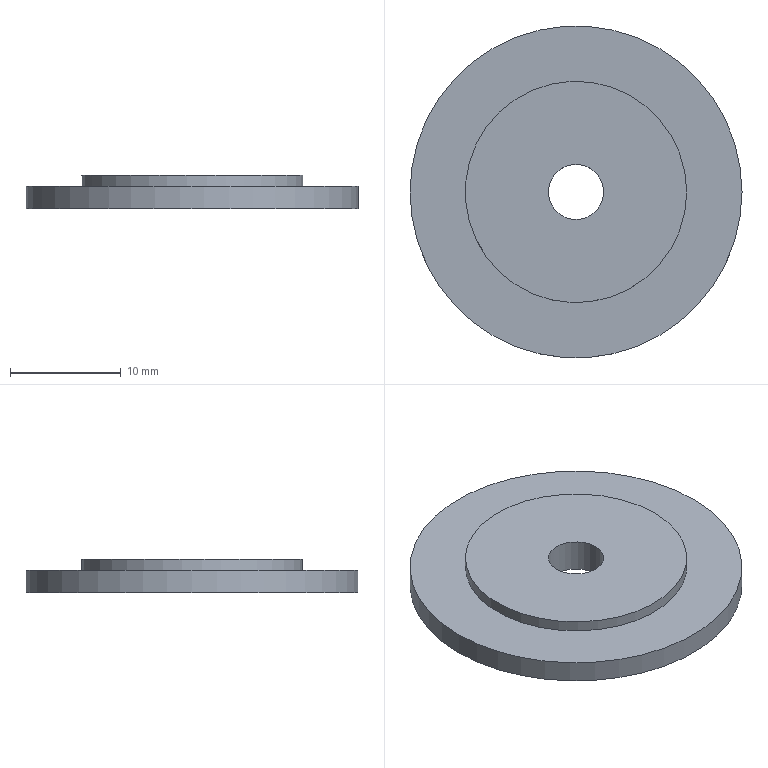Part | NX | features DATUM_CSYS 4, EXTRUDE 3, SKETCH 3 | 1 solid | 6 faces | box 30 x 30 x 3 mm | volume 1669 mm3 | cylinder 3 | plane 3 | commonest cylinder face diameters 5 x1 20 x1 30 x1
STEP:
#1=CARTESIAN_POINT('',(15.,0.,2.));
#2=VERTEX_POINT('',#1);
#3=CARTESIAN_POINT('',(0.,0.,2.));
#4=DIRECTION('',(0.,0.,1.));
#5=DIRECTION('',(1.,0.,0.));
#6=AXIS2_PLACEMENT_3D('',#3,#4,#5);
#7=CIRCLE('',#6,15.);
#8=EDGE_CURVE('',#2,#2,#7,.T.);
#9=ORIENTED_EDGE('',*,*,#8,.F.);
#10=EDGE_LOOP('',(#9));
#11=FACE_BOUND('',#10,.T.);
#12=CARTESIAN_POINT('',(15.,0.,0.));
#13=VERTEX_POINT('',#12);
#14=CARTESIAN_POINT('',(0.,0.,0.));
#15=DIRECTION('',(0.,0.,1.));
#16=DIRECTION('',(1.,0.,0.));
#17=AXIS2_PLACEMENT_3D('',#14,#15,#16);
#18=CIRCLE('',#17,15.);
#19=EDGE_CURVE('',#13,#13,#18,.T.);
#20=ORIENTED_EDGE('',*,*,#19,.T.);
#21=EDGE_LOOP('',(#20));
#22=FACE_BOUND('',#21,.T.);
#23=CARTESIAN_POINT('',(0.,0.,2.));
#24=DIRECTION('',(0.,0.,-1.));
#25=DIRECTION('',(-1.,0.,0.));
#26=AXIS2_PLACEMENT_3D('',#23,#24,#25);
#27=CYLINDRICAL_SURFACE('',#26,15.);
#28=ADVANCED_FACE('',(#11,#22),#27,.T.);
#29=CARTESIAN_POINT('',(10.,0.,2.));
#30=VERTEX_POINT('',#29);
#31=CARTESIAN_POINT('',(0.,0.,2.));
#32=DIRECTION('',(0.,0.,1.));
#33=DIRECTION('',(1.,0.,0.));
#34=AXIS2_PLACEMENT_3D('',#31,#32,#33);
#35=CIRCLE('',#34,10.);
#36=EDGE_CURVE('',#30,#30,#35,.T.);
#37=ORIENTED_EDGE('',*,*,#36,.F.);
#38=EDGE_LOOP('',(#37));
#39=FACE_BOUND('',#38,.T.);
#40=ORIENTED_EDGE('',*,*,#8,.T.);
#41=EDGE_LOOP('',(#40));
#42=FACE_BOUND('',#41,.T.);
#43=CARTESIAN_POINT('',(0.,0.,2.));
#44=DIRECTION('',(0.,0.,1.));
#45=DIRECTION('',(1.,0.,0.));
#46=AXIS2_PLACEMENT_3D('',#43,#44,#45);
#47=PLANE('',#46);
#48=ADVANCED_FACE('',(#39,#42),#47,.T.);
#49=CARTESIAN_POINT('',(2.5,0.,0.));
#50=VERTEX_POINT('',#49);
#51=CARTESIAN_POINT('',(0.,0.,0.));
#52=DIRECTION('',(0.,0.,1.));
#53=DIRECTION('',(1.,0.,0.));
#54=AXIS2_PLACEMENT_3D('',#51,#52,#53);
#55=CIRCLE('',#54,2.5);
#56=EDGE_CURVE('',#50,#50,#55,.T.);
#57=ORIENTED_EDGE('',*,*,#56,.T.);
#58=EDGE_LOOP('',(#57));
#59=FACE_BOUND('',#58,.T.);
#60=ORIENTED_EDGE('',*,*,#19,.F.);
#61=EDGE_LOOP('',(#60));
#62=FACE_BOUND('',#61,.T.);
#63=CARTESIAN_POINT('',(0.,0.,0.));
#64=DIRECTION('',(0.,0.,1.));
#65=DIRECTION('',(1.,0.,0.));
#66=AXIS2_PLACEMENT_3D('',#63,#64,#65);
#67=PLANE('',#66);
#68=ADVANCED_FACE('',(#59,#62),#67,.F.);
#69=ORIENTED_EDGE('',*,*,#56,.F.);
#70=EDGE_LOOP('',(#69));
#71=FACE_BOUND('',#70,.T.);
#72=CARTESIAN_POINT('',(2.5,0.,3.));
#73=VERTEX_POINT('',#72);
#74=CARTESIAN_POINT('',(0.,0.,3.));
#75=DIRECTION('',(0.,0.,1.));
#76=DIRECTION('',(1.,0.,0.));
#77=AXIS2_PLACEMENT_3D('',#74,#75,#76);
#78=CIRCLE('',#77,2.5);
#79=EDGE_CURVE('',#73,#73,#78,.T.);
#80=ORIENTED_EDGE('',*,*,#79,.T.);
#81=EDGE_LOOP('',(#80));
#82=FACE_BOUND('',#81,.T.);
#83=CARTESIAN_POINT('',(0.,0.,0.));
#84=DIRECTION('',(0.,0.,1.));
#85=DIRECTION('',(1.,0.,0.));
#86=AXIS2_PLACEMENT_3D('',#83,#84,#85);
#87=CYLINDRICAL_SURFACE('',#86,2.5);
#88=ADVANCED_FACE('',(#71,#82),#87,.F.);
#89=CARTESIAN_POINT('',(10.,0.,3.));
#90=VERTEX_POINT('',#89);
#91=CARTESIAN_POINT('',(0.,0.,3.));
#92=DIRECTION('',(0.,0.,1.));
#93=DIRECTION('',(1.,0.,0.));
#94=AXIS2_PLACEMENT_3D('',#91,#92,#93);
#95=CIRCLE('',#94,10.);
#96=EDGE_CURVE('',#90,#90,#95,.T.);
#97=ORIENTED_EDGE('',*,*,#96,.F.);
#98=EDGE_LOOP('',(#97));
#99=FACE_BOUND('',#98,.T.);
#100=ORIENTED_EDGE('',*,*,#36,.T.);
#101=EDGE_LOOP('',(#100));
#102=FACE_BOUND('',#101,.T.);
#103=CARTESIAN_POINT('',(0.,0.,3.));
#104=DIRECTION('',(0.,0.,-1.));
#105=DIRECTION('',(-1.,0.,0.));
#106=AXIS2_PLACEMENT_3D('',#103,#104,#105);
#107=CYLINDRICAL_SURFACE('',#106,10.);
#108=ADVANCED_FACE('',(#99,#102),#107,.T.);
#109=ORIENTED_EDGE('',*,*,#96,.T.);
#110=EDGE_LOOP('',(#109));
#111=FACE_BOUND('',#110,.T.);
#112=ORIENTED_EDGE('',*,*,#79,.F.);
#113=EDGE_LOOP('',(#112));
#114=FACE_BOUND('',#113,.T.);
#115=CARTESIAN_POINT('',(0.,0.,3.));
#116=DIRECTION('',(0.,0.,1.));
#117=DIRECTION('',(1.,0.,0.));
#118=AXIS2_PLACEMENT_3D('',#115,#116,#117);
#119=PLANE('',#118);
#120=ADVANCED_FACE('',(#111,#114),#119,.T.);
#121=CLOSED_SHELL('',(#28,#48,#68,#88,#108,#120));
#122=MANIFOLD_SOLID_BREP('',#121);
#123=(LENGTH_UNIT()NAMED_UNIT(*)SI_UNIT(.MILLI.,.METRE.));
#124=UNCERTAINTY_MEASURE_WITH_UNIT(LENGTH_MEASURE(0.00001),#123,'','');
#125=(NAMED_UNIT(*)PLANE_ANGLE_UNIT()SI_UNIT($,.RADIAN.));
#126=(NAMED_UNIT(*)SI_UNIT($,.STERADIAN.)SOLID_ANGLE_UNIT());
#127=(GEOMETRIC_REPRESENTATION_CONTEXT(3)GLOBAL_UNCERTAINTY_ASSIGNED_CONTEXT((#124))GLOBAL_UNIT_ASSIGNED_CONTEXT((#123,#125,#126))REPRESENTATION_CONTEXT('',''));
#128=ADVANCED_BREP_SHAPE_REPRESENTATION('',(#122),#127);